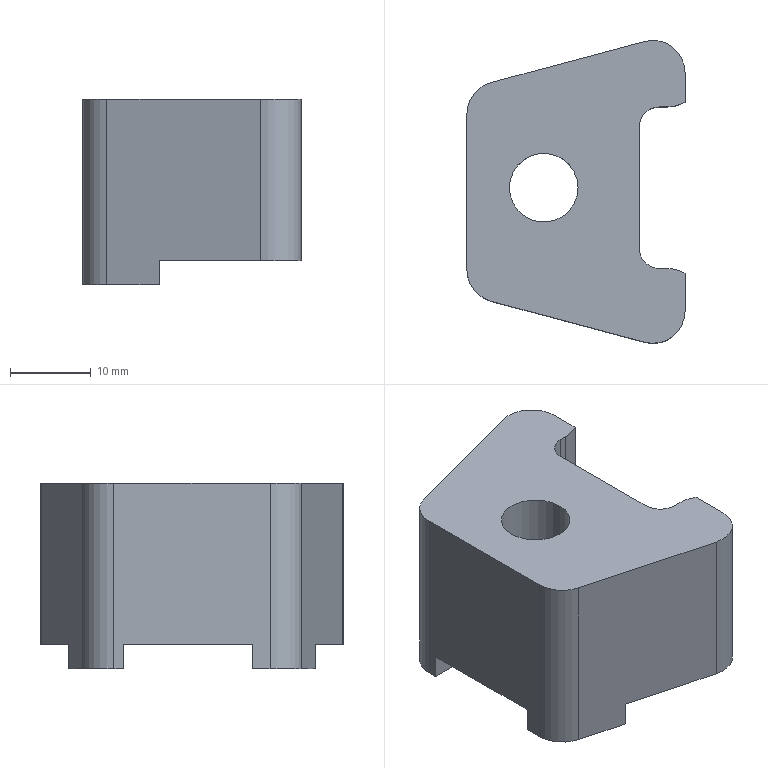Part | NX | features solid 2 | 1 solid | 27 faces | box 27 x 37.502 x 23 mm | volume 13320 mm3 | plane 17 | cylinder 10 | commonest cylinder face diameters 8 x4 5 x2 9 x2 8.5 x1 14 x1
STEP:
#1=CARTESIAN_POINT('',(1518.996,8.,-3.));
#2=VERTEX_POINT('',#1);
#3=CARTESIAN_POINT('',(1518.996,14.736,-3.));
#4=VERTEX_POINT('',#3);
#5=CARTESIAN_POINT('',(1518.996,0.,-3.));
#6=DIRECTION('',(0.,-1.,0.));
#7=VECTOR('',#6,1000.);
#8=LINE('',#5,#7);
#9=EDGE_CURVE('',#2,#4,#8,.F.);
#10=ORIENTED_EDGE('',*,*,#9,.F.);
#11=CARTESIAN_POINT('',(1509.574,8.,-3.));
#12=VERTEX_POINT('',#11);
#13=CARTESIAN_POINT('',(1521.85,8.,-3.));
#14=DIRECTION('',(-1.,0.,0.));
#15=VECTOR('',#14,1000.);
#16=LINE('',#13,#15);
#17=EDGE_CURVE('',#12,#2,#16,.F.);
#18=ORIENTED_EDGE('',*,*,#17,.F.);
#19=CARTESIAN_POINT('',(1509.574,9.142,-3.));
#20=VERTEX_POINT('',#19);
#21=CARTESIAN_POINT('',(1509.574,0.,-3.));
#22=DIRECTION('',(0.,-1.,0.));
#23=VECTOR('',#22,1000.);
#24=LINE('',#21,#23);
#25=EDGE_CURVE('',#12,#20,#24,.F.);
#26=ORIENTED_EDGE('',*,*,#25,.T.);
#27=CARTESIAN_POINT('',(1512.539,13.006,-3.));
#28=VERTEX_POINT('',#27);
#29=CARTESIAN_POINT('',(1513.574,9.142,-3.));
#30=DIRECTION('',(0.,0.,1.));
#31=DIRECTION('',(1.,0.,0.));
#32=AXIS2_PLACEMENT_3D('',#29,#30,#31);
#33=CIRCLE('',#32,4.);
#34=EDGE_CURVE('',#20,#28,#33,.F.);
#35=ORIENTED_EDGE('',*,*,#34,.T.);
#36=CARTESIAN_POINT('',(348.937,-298.78,-3.));
#37=DIRECTION('',(-0.9659,-0.2588,0.));
#38=VECTOR('',#37,1000.);
#39=LINE('',#36,#38);
#40=EDGE_CURVE('',#28,#4,#39,.F.);
#41=ORIENTED_EDGE('',*,*,#40,.T.);
#42=EDGE_LOOP('',(#10,#18,#26,#35,#41));
#43=FACE_BOUND('',#42,.T.);
#44=CARTESIAN_POINT('',(268.879,0.,-3.));
#45=DIRECTION('',(0.,0.,1.));
#46=DIRECTION('',(1.,0.,0.));
#47=AXIS2_PLACEMENT_3D('',#44,#45,#46);
#48=PLANE('',#47);
#49=ADVANCED_FACE('',(#43),#48,.F.);
#50=CARTESIAN_POINT('',(1518.996,-15.771,-3.));
#51=VERTEX_POINT('',#50);
#52=CARTESIAN_POINT('',(1518.996,-8.,-3.));
#53=VERTEX_POINT('',#52);
#54=CARTESIAN_POINT('',(1518.996,0.,-3.));
#55=DIRECTION('',(0.,-1.,0.));
#56=VECTOR('',#55,1000.);
#57=LINE('',#54,#56);
#58=EDGE_CURVE('',#51,#53,#57,.F.);
#59=ORIENTED_EDGE('',*,*,#58,.F.);
#60=CARTESIAN_POINT('',(1512.539,-14.041,-3.));
#61=VERTEX_POINT('',#60);
#62=CARTESIAN_POINT('',(1515.086,-14.724,-3.));
#63=DIRECTION('',(-0.9659,0.2588,0.));
#64=VECTOR('',#63,1000.);
#65=LINE('',#62,#64);
#66=EDGE_CURVE('',#61,#51,#65,.F.);
#67=ORIENTED_EDGE('',*,*,#66,.F.);
#68=CARTESIAN_POINT('',(1509.574,-10.177,-3.));
#69=VERTEX_POINT('',#68);
#70=CARTESIAN_POINT('',(1513.574,-10.177,-3.));
#71=DIRECTION('',(0.,0.,1.));
#72=DIRECTION('',(1.,0.,0.));
#73=AXIS2_PLACEMENT_3D('',#70,#71,#72);
#74=CIRCLE('',#73,4.);
#75=EDGE_CURVE('',#61,#69,#74,.F.);
#76=ORIENTED_EDGE('',*,*,#75,.T.);
#77=CARTESIAN_POINT('',(1509.574,-8.,-3.));
#78=VERTEX_POINT('',#77);
#79=CARTESIAN_POINT('',(1509.574,0.,-3.));
#80=DIRECTION('',(0.,-1.,0.));
#81=VECTOR('',#80,1000.);
#82=LINE('',#79,#81);
#83=EDGE_CURVE('',#69,#78,#82,.F.);
#84=ORIENTED_EDGE('',*,*,#83,.T.);
#85=CARTESIAN_POINT('',(268.879,-8.,-3.));
#86=DIRECTION('',(-1.,0.,0.));
#87=VECTOR('',#86,1000.);
#88=LINE('',#85,#87);
#89=EDGE_CURVE('',#78,#53,#88,.F.);
#90=ORIENTED_EDGE('',*,*,#89,.T.);
#91=EDGE_LOOP('',(#59,#67,#76,#84,#90));
#92=FACE_BOUND('',#91,.T.);
#93=CARTESIAN_POINT('',(268.879,0.,-3.));
#94=DIRECTION('',(0.,0.,1.));
#95=DIRECTION('',(1.,0.,0.));
#96=AXIS2_PLACEMENT_3D('',#93,#94,#95);
#97=PLANE('',#96);
#98=ADVANCED_FACE('',(#92),#97,.F.);
#99=CARTESIAN_POINT('',(1523.324,0.,20.));
#100=VERTEX_POINT('',#99);
#101=CARTESIAN_POINT('',(1519.074,0.,20.));
#102=DIRECTION('',(0.,0.,1.));
#103=DIRECTION('',(1.,0.,0.));
#104=AXIS2_PLACEMENT_3D('',#101,#102,#103);
#105=CIRCLE('',#104,4.25);
#106=EDGE_CURVE('',#100,#100,#105,.T.);
#107=ORIENTED_EDGE('',*,*,#106,.F.);
#108=EDGE_LOOP('',(#107));
#109=FACE_BOUND('',#108,.T.);
#110=CARTESIAN_POINT('',(1534.327,10.,20.));
#111=VERTEX_POINT('',#110);
#112=CARTESIAN_POINT('',(1533.396,10.,20.));
#113=VERTEX_POINT('',#112);
#114=CARTESIAN_POINT('',(1595.285,10.,20.));
#115=DIRECTION('',(1.,0.,0.));
#116=VECTOR('',#115,1000.);
#117=LINE('',#114,#116);
#118=EDGE_CURVE('',#111,#113,#117,.F.);
#119=ORIENTED_EDGE('',*,*,#118,.F.);
#120=CARTESIAN_POINT('',(1536.574,10.601,20.));
#121=VERTEX_POINT('',#120);
#122=CARTESIAN_POINT('',(1534.327,14.5,20.));
#123=DIRECTION('',(0.,0.,1.));
#124=DIRECTION('',(1.,0.,0.));
#125=AXIS2_PLACEMENT_3D('',#122,#123,#124);
#126=CIRCLE('',#125,4.5);
#127=EDGE_CURVE('',#111,#121,#126,.T.);
#128=ORIENTED_EDGE('',*,*,#127,.T.);
#129=CARTESIAN_POINT('',(1536.574,14.233,20.));
#130=VERTEX_POINT('',#129);
#131=CARTESIAN_POINT('',(1536.574,-11.19,20.));
#132=DIRECTION('',(0.,-1.,0.));
#133=VECTOR('',#132,1000.);
#134=LINE('',#131,#133);
#135=EDGE_CURVE('',#130,#121,#134,.T.);
#136=ORIENTED_EDGE('',*,*,#135,.F.);
#137=CARTESIAN_POINT('',(1531.539,18.097,20.));
#138=VERTEX_POINT('',#137);
#139=CARTESIAN_POINT('',(1532.574,14.233,20.));
#140=DIRECTION('',(0.,0.,1.));
#141=DIRECTION('',(1.,0.,0.));
#142=AXIS2_PLACEMENT_3D('',#139,#140,#141);
#143=CIRCLE('',#142,4.);
#144=EDGE_CURVE('',#130,#138,#143,.T.);
#145=ORIENTED_EDGE('',*,*,#144,.T.);
#146=CARTESIAN_POINT('',(1512.539,13.006,20.));
#147=VERTEX_POINT('',#146);
#148=CARTESIAN_POINT('',(1558.853,25.416,20.));
#149=DIRECTION('',(-0.9659,-0.2588,0.));
#150=VECTOR('',#149,1000.);
#151=LINE('',#148,#150);
#152=EDGE_CURVE('',#138,#147,#151,.T.);
#153=ORIENTED_EDGE('',*,*,#152,.T.);
#154=CARTESIAN_POINT('',(1509.574,9.142,20.));
#155=VERTEX_POINT('',#154);
#156=CARTESIAN_POINT('',(1513.574,9.142,20.));
#157=DIRECTION('',(0.,0.,1.));
#158=DIRECTION('',(1.,0.,0.));
#159=AXIS2_PLACEMENT_3D('',#156,#157,#158);
#160=CIRCLE('',#159,4.);
#161=EDGE_CURVE('',#147,#155,#160,.T.);
#162=ORIENTED_EDGE('',*,*,#161,.T.);
#163=CARTESIAN_POINT('',(1509.574,-10.177,20.));
#164=VERTEX_POINT('',#163);
#165=CARTESIAN_POINT('',(1509.574,-7.,20.));
#166=DIRECTION('',(0.,1.,0.));
#167=VECTOR('',#166,1000.);
#168=LINE('',#165,#167);
#169=EDGE_CURVE('',#164,#155,#168,.T.);
#170=ORIENTED_EDGE('',*,*,#169,.F.);
#171=CARTESIAN_POINT('',(1512.539,-14.041,20.));
#172=VERTEX_POINT('',#171);
#173=CARTESIAN_POINT('',(1513.574,-10.177,20.));
#174=DIRECTION('',(0.,0.,1.));
#175=DIRECTION('',(1.,0.,0.));
#176=AXIS2_PLACEMENT_3D('',#173,#174,#175);
#177=CIRCLE('',#176,4.);
#178=EDGE_CURVE('',#164,#172,#177,.T.);
#179=ORIENTED_EDGE('',*,*,#178,.T.);
#180=CARTESIAN_POINT('',(1531.539,-19.132,20.));
#181=VERTEX_POINT('',#180);
#182=CARTESIAN_POINT('',(1613.869,-41.192,20.));
#183=DIRECTION('',(0.9659,-0.2588,0.));
#184=VECTOR('',#183,1000.);
#185=LINE('',#182,#184);
#186=EDGE_CURVE('',#172,#181,#185,.T.);
#187=ORIENTED_EDGE('',*,*,#186,.T.);
#188=CARTESIAN_POINT('',(1536.574,-15.268,20.));
#189=VERTEX_POINT('',#188);
#190=CARTESIAN_POINT('',(1532.574,-15.268,20.));
#191=DIRECTION('',(0.,0.,1.));
#192=DIRECTION('',(1.,0.,0.));
#193=AXIS2_PLACEMENT_3D('',#190,#191,#192);
#194=CIRCLE('',#193,4.);
#195=EDGE_CURVE('',#181,#189,#194,.T.);
#196=ORIENTED_EDGE('',*,*,#195,.T.);
#197=CARTESIAN_POINT('',(1536.574,-10.601,20.));
#198=VERTEX_POINT('',#197);
#199=CARTESIAN_POINT('',(1536.574,-11.19,20.));
#200=DIRECTION('',(0.,-1.,0.));
#201=VECTOR('',#200,1000.);
#202=LINE('',#199,#201);
#203=EDGE_CURVE('',#198,#189,#202,.T.);
#204=ORIENTED_EDGE('',*,*,#203,.F.);
#205=CARTESIAN_POINT('',(1534.327,-10.,20.));
#206=VERTEX_POINT('',#205);
#207=CARTESIAN_POINT('',(1534.327,-14.5,20.));
#208=DIRECTION('',(0.,0.,1.));
#209=DIRECTION('',(1.,0.,0.));
#210=AXIS2_PLACEMENT_3D('',#207,#208,#209);
#211=CIRCLE('',#210,4.5);
#212=EDGE_CURVE('',#198,#206,#211,.T.);
#213=ORIENTED_EDGE('',*,*,#212,.T.);
#214=CARTESIAN_POINT('',(1533.396,-10.,20.));
#215=VERTEX_POINT('',#214);
#216=CARTESIAN_POINT('',(1595.285,-10.,20.));
#217=DIRECTION('',(-1.,0.,0.));
#218=VECTOR('',#217,1000.);
#219=LINE('',#216,#218);
#220=EDGE_CURVE('',#215,#206,#219,.F.);
#221=ORIENTED_EDGE('',*,*,#220,.F.);
#222=CARTESIAN_POINT('',(1530.896,-7.5,20.));
#223=VERTEX_POINT('',#222);
#224=CARTESIAN_POINT('',(1533.396,-7.5,20.));
#225=DIRECTION('',(0.,0.,1.));
#226=DIRECTION('',(1.,0.,0.));
#227=AXIS2_PLACEMENT_3D('',#224,#225,#226);
#228=CIRCLE('',#227,2.5);
#229=EDGE_CURVE('',#223,#215,#228,.T.);
#230=ORIENTED_EDGE('',*,*,#229,.F.);
#231=CARTESIAN_POINT('',(1530.896,7.5,20.));
#232=VERTEX_POINT('',#231);
#233=CARTESIAN_POINT('',(1530.896,-110.548,20.));
#234=DIRECTION('',(0.,-1.,0.));
#235=VECTOR('',#234,1000.);
#236=LINE('',#233,#235);
#237=EDGE_CURVE('',#223,#232,#236,.F.);
#238=ORIENTED_EDGE('',*,*,#237,.T.);
#239=CARTESIAN_POINT('',(1533.396,7.5,20.));
#240=DIRECTION('',(0.,0.,1.));
#241=DIRECTION('',(1.,0.,0.));
#242=AXIS2_PLACEMENT_3D('',#239,#240,#241);
#243=CIRCLE('',#242,2.5);
#244=EDGE_CURVE('',#113,#232,#243,.T.);
#245=ORIENTED_EDGE('',*,*,#244,.F.);
#246=EDGE_LOOP('',(#119,#128,#136,#145,#153,#162,#170,#179,#187,#196,#204,#213,#221,#230,#238,#245));
#247=FACE_BOUND('',#246,.T.);
#248=CARTESIAN_POINT('',(1595.285,-110.548,20.));
#249=DIRECTION('',(0.,0.,1.));
#250=DIRECTION('',(1.,0.,0.));
#251=AXIS2_PLACEMENT_3D('',#248,#249,#250);
#252=PLANE('',#251);
#253=ADVANCED_FACE('',(#109,#247),#252,.T.);
#254=ORIENTED_EDGE('',*,*,#135,.T.);
#255=CARTESIAN_POINT('',(1536.574,10.601,0.));
#256=VERTEX_POINT('',#255);
#257=CARTESIAN_POINT('',(1536.574,10.601,0.));
#258=DIRECTION('',(0.,0.,-1.));
#259=VECTOR('',#258,1000.);
#260=LINE('',#257,#259);
#261=EDGE_CURVE('',#121,#256,#260,.T.);
#262=ORIENTED_EDGE('',*,*,#261,.T.);
#263=CARTESIAN_POINT('',(1536.574,14.233,0.));
#264=VERTEX_POINT('',#263);
#265=CARTESIAN_POINT('',(1536.574,-11.19,0.));
#266=DIRECTION('',(0.,1.,0.));
#267=VECTOR('',#266,1000.);
#268=LINE('',#265,#267);
#269=EDGE_CURVE('',#264,#256,#268,.F.);
#270=ORIENTED_EDGE('',*,*,#269,.F.);
#271=CARTESIAN_POINT('',(1536.574,14.233,-5.));
#272=DIRECTION('',(0.,0.,1.));
#273=VECTOR('',#272,1000.);
#274=LINE('',#271,#273);
#275=EDGE_CURVE('',#264,#130,#274,.T.);
#276=ORIENTED_EDGE('',*,*,#275,.T.);
#277=EDGE_LOOP('',(#254,#262,#270,#276));
#278=FACE_BOUND('',#277,.T.);
#279=CARTESIAN_POINT('',(1536.574,-11.19,-5.));
#280=DIRECTION('',(1.,0.,0.));
#281=DIRECTION('',(0.,0.,-1.));
#282=AXIS2_PLACEMENT_3D('',#279,#280,#281);
#283=PLANE('',#282);
#284=ADVANCED_FACE('',(#278),#283,.T.);
#285=CARTESIAN_POINT('',(1536.574,-10.601,0.));
#286=VERTEX_POINT('',#285);
#287=CARTESIAN_POINT('',(1536.574,-15.268,0.));
#288=VERTEX_POINT('',#287);
#289=CARTESIAN_POINT('',(1536.574,1232.968,0.));
#290=DIRECTION('',(0.,-1.,0.));
#291=VECTOR('',#290,1000.);
#292=LINE('',#289,#291);
#293=EDGE_CURVE('',#286,#288,#292,.T.);
#294=ORIENTED_EDGE('',*,*,#293,.F.);
#295=CARTESIAN_POINT('',(1536.574,-10.601,0.));
#296=DIRECTION('',(0.,0.,-1.));
#297=VECTOR('',#296,1000.);
#298=LINE('',#295,#297);
#299=EDGE_CURVE('',#286,#198,#298,.F.);
#300=ORIENTED_EDGE('',*,*,#299,.T.);
#301=ORIENTED_EDGE('',*,*,#203,.T.);
#302=CARTESIAN_POINT('',(1536.574,-15.268,-5.));
#303=DIRECTION('',(0.,0.,-1.));
#304=VECTOR('',#303,1000.);
#305=LINE('',#302,#304);
#306=EDGE_CURVE('',#189,#288,#305,.T.);
#307=ORIENTED_EDGE('',*,*,#306,.T.);
#308=EDGE_LOOP('',(#294,#300,#301,#307));
#309=FACE_BOUND('',#308,.T.);
#310=CARTESIAN_POINT('',(1536.574,-11.19,-5.));
#311=DIRECTION('',(1.,0.,0.));
#312=DIRECTION('',(0.,0.,-1.));
#313=AXIS2_PLACEMENT_3D('',#310,#311,#312);
#314=PLANE('',#313);
#315=ADVANCED_FACE('',(#309),#314,.T.);
#316=CARTESIAN_POINT('',(1518.996,-8.,0.));
#317=VERTEX_POINT('',#316);
#318=CARTESIAN_POINT('',(1518.996,-8.,-5.));
#319=DIRECTION('',(0.,0.,1.));
#320=VECTOR('',#319,1000.);
#321=LINE('',#318,#320);
#322=EDGE_CURVE('',#53,#317,#321,.T.);
#323=ORIENTED_EDGE('',*,*,#322,.F.);
#324=ORIENTED_EDGE('',*,*,#89,.F.);
#325=CARTESIAN_POINT('',(1509.574,-8.,0.));
#326=VERTEX_POINT('',#325);
#327=CARTESIAN_POINT('',(1509.574,-8.,-5.));
#328=DIRECTION('',(0.,0.,1.));
#329=VECTOR('',#328,1000.);
#330=LINE('',#327,#329);
#331=EDGE_CURVE('',#78,#326,#330,.T.);
#332=ORIENTED_EDGE('',*,*,#331,.T.);
#333=CARTESIAN_POINT('',(1521.85,-8.,0.));
#334=DIRECTION('',(-1.,0.,0.));
#335=VECTOR('',#334,1000.);
#336=LINE('',#333,#335);
#337=EDGE_CURVE('',#317,#326,#336,.T.);
#338=ORIENTED_EDGE('',*,*,#337,.F.);
#339=EDGE_LOOP('',(#323,#324,#332,#338));
#340=FACE_BOUND('',#339,.T.);
#341=CARTESIAN_POINT('',(1521.85,-8.,-5.));
#342=DIRECTION('',(0.,1.,0.));
#343=DIRECTION('',(0.,0.,-1.));
#344=AXIS2_PLACEMENT_3D('',#341,#342,#343);
#345=PLANE('',#344);
#346=ADVANCED_FACE('',(#340),#345,.T.);
#347=CARTESIAN_POINT('',(1518.996,-15.771,0.));
#348=VERTEX_POINT('',#347);
#349=CARTESIAN_POINT('',(1518.996,-15.771,-16.4));
#350=DIRECTION('',(0.,0.,-1.));
#351=VECTOR('',#350,1000.);
#352=LINE('',#349,#351);
#353=EDGE_CURVE('',#348,#51,#352,.T.);
#354=ORIENTED_EDGE('',*,*,#353,.F.);
#355=CARTESIAN_POINT('',(1531.539,-19.132,0.));
#356=VERTEX_POINT('',#355);
#357=CARTESIAN_POINT('',(1515.086,-14.724,0.));
#358=DIRECTION('',(0.9659,-0.2588,0.));
#359=VECTOR('',#358,1000.);
#360=LINE('',#357,#359);
#361=EDGE_CURVE('',#348,#356,#360,.T.);
#362=ORIENTED_EDGE('',*,*,#361,.T.);
#363=CARTESIAN_POINT('',(1531.539,-19.132,-16.4));
#364=DIRECTION('',(0.,0.,-1.));
#365=VECTOR('',#364,1000.);
#366=LINE('',#363,#365);
#367=EDGE_CURVE('',#356,#181,#366,.F.);
#368=ORIENTED_EDGE('',*,*,#367,.T.);
#369=ORIENTED_EDGE('',*,*,#186,.F.);
#370=CARTESIAN_POINT('',(1512.539,-14.041,-16.4));
#371=DIRECTION('',(0.,0.,1.));
#372=VECTOR('',#371,1000.);
#373=LINE('',#370,#372);
#374=EDGE_CURVE('',#172,#61,#373,.F.);
#375=ORIENTED_EDGE('',*,*,#374,.T.);
#376=ORIENTED_EDGE('',*,*,#66,.T.);
#377=EDGE_LOOP('',(#354,#362,#368,#369,#375,#376));
#378=FACE_BOUND('',#377,.T.);
#379=CARTESIAN_POINT('',(1515.086,-14.724,-16.4));
#380=DIRECTION('',(-0.2588,-0.9659,0.));
#381=DIRECTION('',(-0.9659,0.2588,0.));
#382=AXIS2_PLACEMENT_3D('',#379,#380,#381);
#383=PLANE('',#382);
#384=ADVANCED_FACE('',(#378),#383,.T.);
#385=ORIENTED_EDGE('',*,*,#83,.F.);
#386=CARTESIAN_POINT('',(1509.574,-10.177,-5.));
#387=DIRECTION('',(0.,0.,1.));
#388=VECTOR('',#387,1000.);
#389=LINE('',#386,#388);
#390=EDGE_CURVE('',#69,#164,#389,.T.);
#391=ORIENTED_EDGE('',*,*,#390,.T.);
#392=ORIENTED_EDGE('',*,*,#169,.T.);
#393=CARTESIAN_POINT('',(1509.574,9.142,-5.));
#394=DIRECTION('',(0.,0.,-1.));
#395=VECTOR('',#394,1000.);
#396=LINE('',#393,#395);
#397=EDGE_CURVE('',#155,#20,#396,.T.);
#398=ORIENTED_EDGE('',*,*,#397,.T.);
#399=ORIENTED_EDGE('',*,*,#25,.F.);
#400=CARTESIAN_POINT('',(1509.574,8.,0.));
#401=VERTEX_POINT('',#400);
#402=CARTESIAN_POINT('',(1509.574,8.,-5.));
#403=DIRECTION('',(0.,0.,-1.));
#404=VECTOR('',#403,1000.);
#405=LINE('',#402,#404);
#406=EDGE_CURVE('',#401,#12,#405,.T.);
#407=ORIENTED_EDGE('',*,*,#406,.F.);
#408=CARTESIAN_POINT('',(1509.574,1232.968,0.));
#409=DIRECTION('',(0.,1.,0.));
#410=VECTOR('',#409,1000.);
#411=LINE('',#408,#410);
#412=EDGE_CURVE('',#326,#401,#411,.T.);
#413=ORIENTED_EDGE('',*,*,#412,.F.);
#414=ORIENTED_EDGE('',*,*,#331,.F.);
#415=EDGE_LOOP('',(#385,#391,#392,#398,#399,#407,#413,#414));
#416=FACE_BOUND('',#415,.T.);
#417=CARTESIAN_POINT('',(1509.574,-7.,-5.));
#418=DIRECTION('',(-1.,0.,0.));
#419=DIRECTION('',(0.,0.,1.));
#420=AXIS2_PLACEMENT_3D('',#417,#418,#419);
#421=PLANE('',#420);
#422=ADVANCED_FACE('',(#416),#421,.T.);
#423=CARTESIAN_POINT('',(1518.996,8.,0.));
#424=VERTEX_POINT('',#423);
#425=CARTESIAN_POINT('',(1518.996,8.,-5.));
#426=DIRECTION('',(0.,0.,-1.));
#427=VECTOR('',#426,1000.);
#428=LINE('',#425,#427);
#429=EDGE_CURVE('',#424,#2,#428,.T.);
#430=ORIENTED_EDGE('',*,*,#429,.F.);
#431=CARTESIAN_POINT('',(1521.85,8.,0.));
#432=DIRECTION('',(1.,0.,0.));
#433=VECTOR('',#432,1000.);
#434=LINE('',#431,#433);
#435=EDGE_CURVE('',#401,#424,#434,.T.);
#436=ORIENTED_EDGE('',*,*,#435,.F.);
#437=ORIENTED_EDGE('',*,*,#406,.T.);
#438=ORIENTED_EDGE('',*,*,#17,.T.);
#439=EDGE_LOOP('',(#430,#436,#437,#438));
#440=FACE_BOUND('',#439,.T.);
#441=CARTESIAN_POINT('',(1521.85,8.,-5.));
#442=DIRECTION('',(0.,-1.,0.));
#443=DIRECTION('',(0.,0.,-1.));
#444=AXIS2_PLACEMENT_3D('',#441,#442,#443);
#445=PLANE('',#444);
#446=ADVANCED_FACE('',(#440),#445,.T.);
#447=CARTESIAN_POINT('',(1518.996,14.736,0.));
#448=VERTEX_POINT('',#447);
#449=CARTESIAN_POINT('',(1518.996,14.736,-16.4));
#450=DIRECTION('',(0.,0.,1.));
#451=VECTOR('',#450,1000.);
#452=LINE('',#449,#451);
#453=EDGE_CURVE('',#4,#448,#452,.T.);
#454=ORIENTED_EDGE('',*,*,#453,.F.);
#455=ORIENTED_EDGE('',*,*,#40,.F.);
#456=CARTESIAN_POINT('',(1512.539,13.006,-16.4));
#457=DIRECTION('',(0.,0.,-1.));
#458=VECTOR('',#457,1000.);
#459=LINE('',#456,#458);
#460=EDGE_CURVE('',#28,#147,#459,.F.);
#461=ORIENTED_EDGE('',*,*,#460,.T.);
#462=ORIENTED_EDGE('',*,*,#152,.F.);
#463=CARTESIAN_POINT('',(1531.539,18.097,0.));
#464=VERTEX_POINT('',#463);
#465=CARTESIAN_POINT('',(1531.539,18.097,-16.4));
#466=DIRECTION('',(0.,0.,1.));
#467=VECTOR('',#466,1000.);
#468=LINE('',#465,#467);
#469=EDGE_CURVE('',#138,#464,#468,.F.);
#470=ORIENTED_EDGE('',*,*,#469,.T.);
#471=CARTESIAN_POINT('',(942.381,-139.768,0.));
#472=DIRECTION('',(0.9659,0.2588,0.));
#473=VECTOR('',#472,1000.);
#474=LINE('',#471,#473);
#475=EDGE_CURVE('',#448,#464,#474,.T.);
#476=ORIENTED_EDGE('',*,*,#475,.F.);
#477=EDGE_LOOP('',(#454,#455,#461,#462,#470,#476));
#478=FACE_BOUND('',#477,.T.);
#479=CARTESIAN_POINT('',(1515.345,13.758,-16.4));
#480=DIRECTION('',(-0.2588,0.9659,0.));
#481=DIRECTION('',(-0.9659,-0.2588,0.));
#482=AXIS2_PLACEMENT_3D('',#479,#480,#481);
#483=PLANE('',#482);
#484=ADVANCED_FACE('',(#478),#483,.T.);
#485=CARTESIAN_POINT('',(1518.996,1232.968,0.));
#486=DIRECTION('',(0.,1.,0.));
#487=VECTOR('',#486,1000.);
#488=LINE('',#485,#487);
#489=EDGE_CURVE('',#448,#424,#488,.F.);
#490=ORIENTED_EDGE('',*,*,#489,.F.);
#491=ORIENTED_EDGE('',*,*,#475,.T.);
#492=CARTESIAN_POINT('',(1532.574,14.233,0.));
#493=DIRECTION('',(0.,0.,-1.));
#494=DIRECTION('',(-1.,0.,0.));
#495=AXIS2_PLACEMENT_3D('',#492,#493,#494);
#496=CIRCLE('',#495,4.);
#497=EDGE_CURVE('',#464,#264,#496,.T.);
#498=ORIENTED_EDGE('',*,*,#497,.T.);
#499=ORIENTED_EDGE('',*,*,#269,.T.);
#500=CARTESIAN_POINT('',(1534.327,10.,0.));
#501=VERTEX_POINT('',#500);
#502=CARTESIAN_POINT('',(1534.327,14.5,0.));
#503=DIRECTION('',(0.,0.,-1.));
#504=DIRECTION('',(-1.,0.,0.));
#505=AXIS2_PLACEMENT_3D('',#502,#503,#504);
#506=CIRCLE('',#505,4.5);
#507=EDGE_CURVE('',#256,#501,#506,.T.);
#508=ORIENTED_EDGE('',*,*,#507,.T.);
#509=CARTESIAN_POINT('',(1533.396,10.,0.));
#510=VERTEX_POINT('',#509);
#511=CARTESIAN_POINT('',(574.557,10.,0.));
#512=DIRECTION('',(-1.,0.,0.));
#513=VECTOR('',#512,1000.);
#514=LINE('',#511,#513);
#515=EDGE_CURVE('',#510,#501,#514,.F.);
#516=ORIENTED_EDGE('',*,*,#515,.F.);
#517=CARTESIAN_POINT('',(1530.896,7.5,0.));
#518=VERTEX_POINT('',#517);
#519=CARTESIAN_POINT('',(1533.396,7.5,0.));
#520=DIRECTION('',(0.,0.,-1.));
#521=DIRECTION('',(-1.,0.,0.));
#522=AXIS2_PLACEMENT_3D('',#519,#520,#521);
#523=CIRCLE('',#522,2.5);
#524=EDGE_CURVE('',#518,#510,#523,.T.);
#525=ORIENTED_EDGE('',*,*,#524,.F.);
#526=CARTESIAN_POINT('',(1530.896,-7.5,0.));
#527=VERTEX_POINT('',#526);
#528=CARTESIAN_POINT('',(1530.896,1232.968,0.));
#529=DIRECTION('',(0.,1.,0.));
#530=VECTOR('',#529,1000.);
#531=LINE('',#528,#530);
#532=EDGE_CURVE('',#518,#527,#531,.F.);
#533=ORIENTED_EDGE('',*,*,#532,.T.);
#534=CARTESIAN_POINT('',(1533.396,-10.,0.));
#535=VERTEX_POINT('',#534);
#536=CARTESIAN_POINT('',(1533.396,-7.5,0.));
#537=DIRECTION('',(0.,0.,-1.));
#538=DIRECTION('',(-1.,0.,0.));
#539=AXIS2_PLACEMENT_3D('',#536,#537,#538);
#540=CIRCLE('',#539,2.5);
#541=EDGE_CURVE('',#535,#527,#540,.T.);
#542=ORIENTED_EDGE('',*,*,#541,.F.);
#543=CARTESIAN_POINT('',(1534.327,-10.,0.));
#544=VERTEX_POINT('',#543);
#545=CARTESIAN_POINT('',(574.557,-10.,0.));
#546=DIRECTION('',(1.,0.,0.));
#547=VECTOR('',#546,1000.);
#548=LINE('',#545,#547);
#549=EDGE_CURVE('',#544,#535,#548,.F.);
#550=ORIENTED_EDGE('',*,*,#549,.F.);
#551=CARTESIAN_POINT('',(1534.327,-14.5,0.));
#552=DIRECTION('',(0.,0.,-1.));
#553=DIRECTION('',(-1.,0.,0.));
#554=AXIS2_PLACEMENT_3D('',#551,#552,#553);
#555=CIRCLE('',#554,4.5);
#556=EDGE_CURVE('',#544,#286,#555,.T.);
#557=ORIENTED_EDGE('',*,*,#556,.T.);
#558=ORIENTED_EDGE('',*,*,#293,.T.);
#559=CARTESIAN_POINT('',(1532.574,-15.268,0.));
#560=DIRECTION('',(0.,0.,-1.));
#561=DIRECTION('',(-1.,0.,0.));
#562=AXIS2_PLACEMENT_3D('',#559,#560,#561);
#563=CIRCLE('',#562,4.);
#564=EDGE_CURVE('',#288,#356,#563,.T.);
#565=ORIENTED_EDGE('',*,*,#564,.T.);
#566=ORIENTED_EDGE('',*,*,#361,.F.);
#567=CARTESIAN_POINT('',(1518.996,1232.968,0.));
#568=DIRECTION('',(0.,1.,0.));
#569=VECTOR('',#568,1000.);
#570=LINE('',#567,#569);
#571=EDGE_CURVE('',#317,#348,#570,.F.);
#572=ORIENTED_EDGE('',*,*,#571,.F.);
#573=ORIENTED_EDGE('',*,*,#337,.T.);
#574=ORIENTED_EDGE('',*,*,#412,.T.);
#575=ORIENTED_EDGE('',*,*,#435,.T.);
#576=EDGE_LOOP('',(#490,#491,#498,#499,#508,#516,#525,#533,#542,#550,#557,#558,#565,#566,#572,#573,#574,#575));
#577=FACE_BOUND('',#576,.T.);
#578=CARTESIAN_POINT('',(1512.074,0.,0.));
#579=VERTEX_POINT('',#578);
#580=CARTESIAN_POINT('',(1519.074,0.,0.));
#581=DIRECTION('',(0.,0.,-1.));
#582=DIRECTION('',(-1.,0.,0.));
#583=AXIS2_PLACEMENT_3D('',#580,#581,#582);
#584=CIRCLE('',#583,7.);
#585=EDGE_CURVE('',#579,#579,#584,.F.);
#586=ORIENTED_EDGE('',*,*,#585,.T.);
#587=EDGE_LOOP('',(#586));
#588=FACE_BOUND('',#587,.T.);
#589=CARTESIAN_POINT('',(574.557,1232.968,0.));
#590=DIRECTION('',(0.,0.,-1.));
#591=DIRECTION('',(-0.9659,0.2588,0.));
#592=AXIS2_PLACEMENT_3D('',#589,#590,#591);
#593=PLANE('',#592);
#594=ADVANCED_FACE('',(#577,#588),#593,.T.);
#595=ORIENTED_EDGE('',*,*,#178,.F.);
#596=ORIENTED_EDGE('',*,*,#390,.F.);
#597=ORIENTED_EDGE('',*,*,#75,.F.);
#598=ORIENTED_EDGE('',*,*,#374,.F.);
#599=EDGE_LOOP('',(#595,#596,#597,#598));
#600=FACE_BOUND('',#599,.T.);
#601=CARTESIAN_POINT('',(1513.574,-10.177,-5.));
#602=DIRECTION('',(0.,0.,1.));
#603=DIRECTION('',(1.,0.,0.));
#604=AXIS2_PLACEMENT_3D('',#601,#602,#603);
#605=CYLINDRICAL_SURFACE('',#604,4.);
#606=ADVANCED_FACE('',(#600),#605,.T.);
#607=ORIENTED_EDGE('',*,*,#34,.F.);
#608=ORIENTED_EDGE('',*,*,#397,.F.);
#609=ORIENTED_EDGE('',*,*,#161,.F.);
#610=ORIENTED_EDGE('',*,*,#460,.F.);
#611=EDGE_LOOP('',(#607,#608,#609,#610));
#612=FACE_BOUND('',#611,.T.);
#613=CARTESIAN_POINT('',(1513.574,9.142,-5.));
#614=DIRECTION('',(0.,0.,-1.));
#615=DIRECTION('',(-1.,0.,0.));
#616=AXIS2_PLACEMENT_3D('',#613,#614,#615);
#617=CYLINDRICAL_SURFACE('',#616,4.);
#618=ADVANCED_FACE('',(#612),#617,.T.);
#619=ORIENTED_EDGE('',*,*,#106,.T.);
#620=EDGE_LOOP('',(#619));
#621=FACE_BOUND('',#620,.T.);
#622=CARTESIAN_POINT('',(1523.324,0.,10.));
#623=VERTEX_POINT('',#622);
#624=CARTESIAN_POINT('',(1519.074,0.,10.));
#625=DIRECTION('',(0.,0.,1.));
#626=DIRECTION('',(1.,0.,0.));
#627=AXIS2_PLACEMENT_3D('',#624,#625,#626);
#628=CIRCLE('',#627,4.25);
#629=EDGE_CURVE('',#623,#623,#628,.F.);
#630=ORIENTED_EDGE('',*,*,#629,.T.);
#631=EDGE_LOOP('',(#630));
#632=FACE_BOUND('',#631,.T.);
#633=CARTESIAN_POINT('',(1519.074,0.,50.));
#634=DIRECTION('',(0.,0.,1.));
#635=DIRECTION('',(1.,0.,0.));
#636=AXIS2_PLACEMENT_3D('',#633,#634,#635);
#637=CYLINDRICAL_SURFACE('',#636,4.25);
#638=ADVANCED_FACE('',(#621,#632),#637,.F.);
#639=ORIENTED_EDGE('',*,*,#629,.F.);
#640=EDGE_LOOP('',(#639));
#641=FACE_BOUND('',#640,.T.);
#642=CARTESIAN_POINT('',(1526.074,0.,10.));
#643=VERTEX_POINT('',#642);
#644=CARTESIAN_POINT('',(1519.074,0.,10.));
#645=DIRECTION('',(0.,0.,1.));
#646=DIRECTION('',(1.,0.,0.));
#647=AXIS2_PLACEMENT_3D('',#644,#645,#646);
#648=CIRCLE('',#647,7.);
#649=EDGE_CURVE('',#643,#643,#648,.F.);
#650=ORIENTED_EDGE('',*,*,#649,.T.);
#651=EDGE_LOOP('',(#650));
#652=FACE_BOUND('',#651,.T.);
#653=CARTESIAN_POINT('',(1519.074,0.,10.));
#654=DIRECTION('',(0.,0.,1.));
#655=DIRECTION('',(1.,0.,0.));
#656=AXIS2_PLACEMENT_3D('',#653,#654,#655);
#657=PLANE('',#656);
#658=ADVANCED_FACE('',(#641,#652),#657,.F.);
#659=ORIENTED_EDGE('',*,*,#649,.F.);
#660=EDGE_LOOP('',(#659));
#661=FACE_BOUND('',#660,.T.);
#662=ORIENTED_EDGE('',*,*,#585,.F.);
#663=EDGE_LOOP('',(#662));
#664=FACE_BOUND('',#663,.T.);
#665=CARTESIAN_POINT('',(1519.074,0.,0.));
#666=DIRECTION('',(0.,0.,1.));
#667=DIRECTION('',(1.,0.,0.));
#668=AXIS2_PLACEMENT_3D('',#665,#666,#667);
#669=CYLINDRICAL_SURFACE('',#668,7.);
#670=ADVANCED_FACE('',(#661,#664),#669,.F.);
#671=ORIENTED_EDGE('',*,*,#367,.F.);
#672=ORIENTED_EDGE('',*,*,#564,.F.);
#673=ORIENTED_EDGE('',*,*,#306,.F.);
#674=ORIENTED_EDGE('',*,*,#195,.F.);
#675=EDGE_LOOP('',(#671,#672,#673,#674));
#676=FACE_BOUND('',#675,.T.);
#677=CARTESIAN_POINT('',(1532.574,-15.268,-5.));
#678=DIRECTION('',(0.,0.,-1.));
#679=DIRECTION('',(-1.,0.,0.));
#680=AXIS2_PLACEMENT_3D('',#677,#678,#679);
#681=CYLINDRICAL_SURFACE('',#680,4.);
#682=ADVANCED_FACE('',(#676),#681,.T.);
#683=ORIENTED_EDGE('',*,*,#497,.F.);
#684=ORIENTED_EDGE('',*,*,#469,.F.);
#685=ORIENTED_EDGE('',*,*,#144,.F.);
#686=ORIENTED_EDGE('',*,*,#275,.F.);
#687=EDGE_LOOP('',(#683,#684,#685,#686));
#688=FACE_BOUND('',#687,.T.);
#689=CARTESIAN_POINT('',(1532.574,14.233,-5.));
#690=DIRECTION('',(0.,0.,1.));
#691=DIRECTION('',(1.,0.,0.));
#692=AXIS2_PLACEMENT_3D('',#689,#690,#691);
#693=CYLINDRICAL_SURFACE('',#692,4.);
#694=ADVANCED_FACE('',(#688),#693,.T.);
#695=CARTESIAN_POINT('',(1534.327,10.,0.));
#696=DIRECTION('',(0.,0.,1.));
#697=VECTOR('',#696,1000.);
#698=LINE('',#695,#697);
#699=EDGE_CURVE('',#501,#111,#698,.T.);
#700=ORIENTED_EDGE('',*,*,#699,.F.);
#701=ORIENTED_EDGE('',*,*,#507,.F.);
#702=ORIENTED_EDGE('',*,*,#261,.F.);
#703=ORIENTED_EDGE('',*,*,#127,.F.);
#704=EDGE_LOOP('',(#700,#701,#702,#703));
#705=FACE_BOUND('',#704,.T.);
#706=CARTESIAN_POINT('',(1534.327,14.5,0.));
#707=DIRECTION('',(0.,0.,-1.));
#708=DIRECTION('',(-1.,0.,0.));
#709=AXIS2_PLACEMENT_3D('',#706,#707,#708);
#710=CYLINDRICAL_SURFACE('',#709,4.5);
#711=ADVANCED_FACE('',(#705),#710,.T.);
#712=ORIENTED_EDGE('',*,*,#118,.T.);
#713=CARTESIAN_POINT('',(1533.396,10.,0.));
#714=DIRECTION('',(0.,0.,1.));
#715=VECTOR('',#714,1000.);
#716=LINE('',#713,#715);
#717=EDGE_CURVE('',#113,#510,#716,.F.);
#718=ORIENTED_EDGE('',*,*,#717,.T.);
#719=ORIENTED_EDGE('',*,*,#515,.T.);
#720=ORIENTED_EDGE('',*,*,#699,.T.);
#721=EDGE_LOOP('',(#712,#718,#719,#720));
#722=FACE_BOUND('',#721,.T.);
#723=CARTESIAN_POINT('',(984.466,10.,0.));
#724=DIRECTION('',(0.,-1.,0.));
#725=DIRECTION('',(1.,0.,0.));
#726=AXIS2_PLACEMENT_3D('',#723,#724,#725);
#727=PLANE('',#726);
#728=ADVANCED_FACE('',(#722),#727,.T.);
#729=ORIENTED_EDGE('',*,*,#524,.T.);
#730=ORIENTED_EDGE('',*,*,#717,.F.);
#731=ORIENTED_EDGE('',*,*,#244,.T.);
#732=CARTESIAN_POINT('',(1530.896,7.5,0.));
#733=DIRECTION('',(0.,0.,1.));
#734=VECTOR('',#733,1000.);
#735=LINE('',#732,#734);
#736=EDGE_CURVE('',#518,#232,#735,.T.);
#737=ORIENTED_EDGE('',*,*,#736,.F.);
#738=EDGE_LOOP('',(#729,#730,#731,#737));
#739=FACE_BOUND('',#738,.T.);
#740=CARTESIAN_POINT('',(1533.396,7.5,0.));
#741=DIRECTION('',(0.,0.,1.));
#742=DIRECTION('',(1.,0.,0.));
#743=AXIS2_PLACEMENT_3D('',#740,#741,#742);
#744=CYLINDRICAL_SURFACE('',#743,2.5);
#745=ADVANCED_FACE('',(#739),#744,.F.);
#746=CARTESIAN_POINT('',(1530.896,-7.5,0.));
#747=DIRECTION('',(0.,0.,1.));
#748=VECTOR('',#747,1000.);
#749=LINE('',#746,#748);
#750=EDGE_CURVE('',#527,#223,#749,.T.);
#751=ORIENTED_EDGE('',*,*,#750,.F.);
#752=ORIENTED_EDGE('',*,*,#532,.F.);
#753=ORIENTED_EDGE('',*,*,#736,.T.);
#754=ORIENTED_EDGE('',*,*,#237,.F.);
#755=EDGE_LOOP('',(#751,#752,#753,#754));
#756=FACE_BOUND('',#755,.T.);
#757=CARTESIAN_POINT('',(1530.896,0.,0.));
#758=DIRECTION('',(-1.,0.,0.));
#759=DIRECTION('',(0.,-1.,0.));
#760=AXIS2_PLACEMENT_3D('',#757,#758,#759);
#761=PLANE('',#760);
#762=ADVANCED_FACE('',(#756),#761,.F.);
#763=CARTESIAN_POINT('',(1533.396,-10.,0.));
#764=DIRECTION('',(0.,0.,1.));
#765=VECTOR('',#764,1000.);
#766=LINE('',#763,#765);
#767=EDGE_CURVE('',#215,#535,#766,.F.);
#768=ORIENTED_EDGE('',*,*,#767,.T.);
#769=ORIENTED_EDGE('',*,*,#541,.T.);
#770=ORIENTED_EDGE('',*,*,#750,.T.);
#771=ORIENTED_EDGE('',*,*,#229,.T.);
#772=EDGE_LOOP('',(#768,#769,#770,#771));
#773=FACE_BOUND('',#772,.T.);
#774=CARTESIAN_POINT('',(1533.396,-7.5,0.));
#775=DIRECTION('',(0.,0.,1.));
#776=DIRECTION('',(1.,0.,0.));
#777=AXIS2_PLACEMENT_3D('',#774,#775,#776);
#778=CYLINDRICAL_SURFACE('',#777,2.5);
#779=ADVANCED_FACE('',(#773),#778,.F.);
#780=ORIENTED_EDGE('',*,*,#220,.T.);
#781=CARTESIAN_POINT('',(1534.327,-10.,0.));
#782=DIRECTION('',(0.,0.,-1.));
#783=VECTOR('',#782,1000.);
#784=LINE('',#781,#783);
#785=EDGE_CURVE('',#544,#206,#784,.F.);
#786=ORIENTED_EDGE('',*,*,#785,.F.);
#787=ORIENTED_EDGE('',*,*,#549,.T.);
#788=ORIENTED_EDGE('',*,*,#767,.F.);
#789=EDGE_LOOP('',(#780,#786,#787,#788));
#790=FACE_BOUND('',#789,.T.);
#791=CARTESIAN_POINT('',(984.466,-10.,0.));
#792=DIRECTION('',(0.,1.,0.));
#793=DIRECTION('',(1.,0.,0.));
#794=AXIS2_PLACEMENT_3D('',#791,#792,#793);
#795=PLANE('',#794);
#796=ADVANCED_FACE('',(#790),#795,.T.);
#797=ORIENTED_EDGE('',*,*,#299,.F.);
#798=ORIENTED_EDGE('',*,*,#556,.F.);
#799=ORIENTED_EDGE('',*,*,#785,.T.);
#800=ORIENTED_EDGE('',*,*,#212,.F.);
#801=EDGE_LOOP('',(#797,#798,#799,#800));
#802=FACE_BOUND('',#801,.T.);
#803=CARTESIAN_POINT('',(1534.327,-14.5,0.));
#804=DIRECTION('',(0.,0.,-1.));
#805=DIRECTION('',(-1.,0.,0.));
#806=AXIS2_PLACEMENT_3D('',#803,#804,#805);
#807=CYLINDRICAL_SURFACE('',#806,4.5);
#808=ADVANCED_FACE('',(#802),#807,.T.);
#809=ORIENTED_EDGE('',*,*,#429,.T.);
#810=ORIENTED_EDGE('',*,*,#9,.T.);
#811=ORIENTED_EDGE('',*,*,#453,.T.);
#812=ORIENTED_EDGE('',*,*,#489,.T.);
#813=EDGE_LOOP('',(#809,#810,#811,#812));
#814=FACE_BOUND('',#813,.T.);
#815=CARTESIAN_POINT('',(1518.996,-0.455,-6.));
#816=DIRECTION('',(-1.,0.,0.));
#817=DIRECTION('',(0.,0.,1.));
#818=AXIS2_PLACEMENT_3D('',#815,#816,#817);
#819=PLANE('',#818);
#820=ADVANCED_FACE('',(#814),#819,.F.);
#821=ORIENTED_EDGE('',*,*,#322,.T.);
#822=ORIENTED_EDGE('',*,*,#571,.T.);
#823=ORIENTED_EDGE('',*,*,#353,.T.);
#824=ORIENTED_EDGE('',*,*,#58,.T.);
#825=EDGE_LOOP('',(#821,#822,#823,#824));
#826=FACE_BOUND('',#825,.T.);
#827=CARTESIAN_POINT('',(1518.996,-0.455,-6.));
#828=DIRECTION('',(-1.,0.,0.));
#829=DIRECTION('',(0.,0.,1.));
#830=AXIS2_PLACEMENT_3D('',#827,#828,#829);
#831=PLANE('',#830);
#832=ADVANCED_FACE('',(#826),#831,.F.);
#833=CLOSED_SHELL('',(#49,#98,#253,#284,#315,#346,#384,#422,#446,#484,#594,#606,#618,#638,#658,#670,#682,#694,#711,#728,#745,#762,#779,#796,#808,#820,#832));
#834=MANIFOLD_SOLID_BREP('',#833);
#835=(LENGTH_UNIT()NAMED_UNIT(*)SI_UNIT(.MILLI.,.METRE.));
#836=UNCERTAINTY_MEASURE_WITH_UNIT(LENGTH_MEASURE(0.00001),#835,'','');
#837=(NAMED_UNIT(*)PLANE_ANGLE_UNIT()SI_UNIT($,.RADIAN.));
#838=(NAMED_UNIT(*)SI_UNIT($,.STERADIAN.)SOLID_ANGLE_UNIT());
#839=(GEOMETRIC_REPRESENTATION_CONTEXT(3)GLOBAL_UNCERTAINTY_ASSIGNED_CONTEXT((#836))GLOBAL_UNIT_ASSIGNED_CONTEXT((#835,#837,#838))REPRESENTATION_CONTEXT('',''));
#840=ADVANCED_BREP_SHAPE_REPRESENTATION('',(#834),#839);